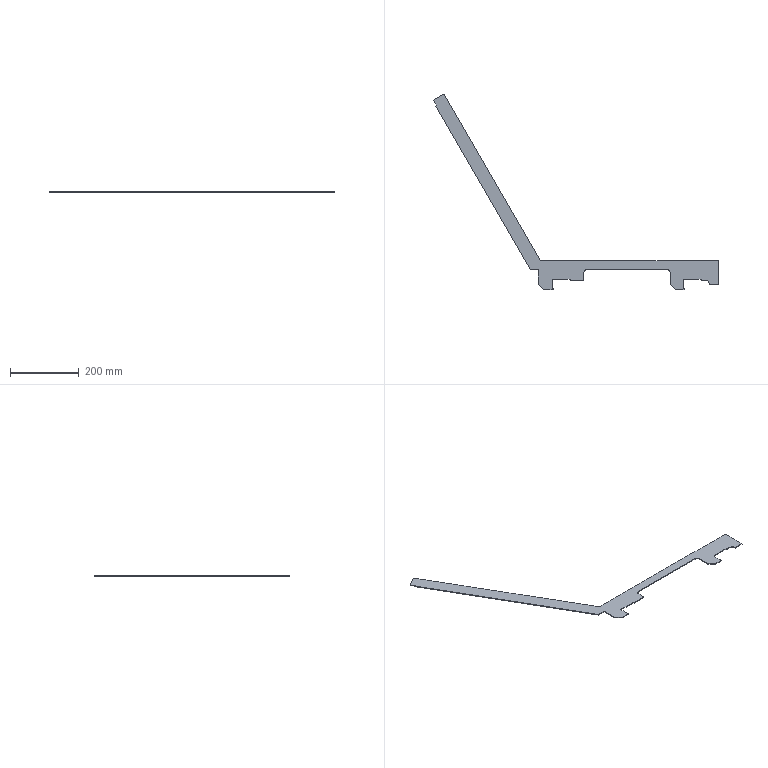Part | STEP file | zq001-1 | 1 solid | 37 faces | box 827.736 x 568.376 x 2 mm | volume 90659 mm3 | plane 32 | cylinder 5 | commonest cylinder face diameters 20 x3 2 x2
STEP:
#1=CARTESIAN_POINT('',(-553.217,491.842,-2.));
#2=VERTEX_POINT('',#1);
#3=CARTESIAN_POINT('',(-544.917,477.466,-2.));
#4=VERTEX_POINT('',#3);
#5=CARTESIAN_POINT('',(-553.217,491.842,-2.));
#6=DIRECTION('',(0.5,-0.866,0.));
#7=VECTOR('',#6,1000.);
#8=LINE('',#5,#7);
#9=EDGE_CURVE('',#2,#4,#8,.T.);
#10=ORIENTED_EDGE('',*,*,#9,.F.);
#11=CARTESIAN_POINT('',(-523.079,509.242,-2.));
#12=VERTEX_POINT('',#11);
#13=CARTESIAN_POINT('',(-523.079,509.242,-2.));
#14=DIRECTION('',(-0.866,-0.5,0.));
#15=VECTOR('',#14,1000.);
#16=LINE('',#13,#15);
#17=EDGE_CURVE('',#12,#2,#16,.T.);
#18=ORIENTED_EDGE('',*,*,#17,.F.);
#19=CARTESIAN_POINT('',(-521.713,508.876,-2.));
#20=VERTEX_POINT('',#19);
#21=CARTESIAN_POINT('',(-522.579,508.376,-2.));
#22=DIRECTION('',(0.,0.,1.));
#23=DIRECTION('',(1.,0.,0.));
#24=AXIS2_PLACEMENT_3D('',#21,#22,#23);
#25=CIRCLE('',#24,1.);
#26=EDGE_CURVE('',#20,#12,#25,.T.);
#27=ORIENTED_EDGE('',*,*,#26,.F.);
#28=CARTESIAN_POINT('',(-242.636,25.5,-2.));
#29=VERTEX_POINT('',#28);
#30=CARTESIAN_POINT('',(-242.636,25.5,-2.));
#31=DIRECTION('',(-0.5,0.866,0.));
#32=VECTOR('',#31,1000.);
#33=LINE('',#30,#32);
#34=EDGE_CURVE('',#29,#20,#33,.T.);
#35=ORIENTED_EDGE('',*,*,#34,.F.);
#36=CARTESIAN_POINT('',(273.519,25.5,-2.));
#37=VERTEX_POINT('',#36);
#38=CARTESIAN_POINT('',(-522.579,25.5,-2.));
#39=DIRECTION('',(-1.,0.,0.));
#40=VECTOR('',#39,1000.);
#41=LINE('',#38,#40);
#42=EDGE_CURVE('',#37,#29,#41,.T.);
#43=ORIENTED_EDGE('',*,*,#42,.F.);
#44=CARTESIAN_POINT('',(274.519,24.5,-2.));
#45=VERTEX_POINT('',#44);
#46=CARTESIAN_POINT('',(273.519,24.5,-2.));
#47=DIRECTION('',(0.,0.,1.));
#48=DIRECTION('',(1.,0.,0.));
#49=AXIS2_PLACEMENT_3D('',#46,#47,#48);
#50=CIRCLE('',#49,1.);
#51=EDGE_CURVE('',#45,#37,#50,.T.);
#52=ORIENTED_EDGE('',*,*,#51,.F.);
#53=CARTESIAN_POINT('',(274.519,-42.5,-2.));
#54=VERTEX_POINT('',#53);
#55=CARTESIAN_POINT('',(274.519,508.376,-2.));
#56=DIRECTION('',(0.,1.,0.));
#57=VECTOR('',#56,1000.);
#58=LINE('',#55,#57);
#59=EDGE_CURVE('',#54,#45,#58,.T.);
#60=ORIENTED_EDGE('',*,*,#59,.F.);
#61=CARTESIAN_POINT('',(246.519,-42.5,-2.));
#62=VERTEX_POINT('',#61);
#63=CARTESIAN_POINT('',(-522.579,-42.5,-2.));
#64=DIRECTION('',(1.,0.,0.));
#65=VECTOR('',#64,1000.);
#66=LINE('',#63,#65);
#67=EDGE_CURVE('',#62,#54,#66,.T.);
#68=ORIENTED_EDGE('',*,*,#67,.F.);
#69=CARTESIAN_POINT('',(246.519,-40.5,-2.));
#70=VERTEX_POINT('',#69);
#71=CARTESIAN_POINT('',(246.519,508.376,-2.));
#72=DIRECTION('',(0.,-1.,0.));
#73=VECTOR('',#72,1000.);
#74=LINE('',#71,#73);
#75=EDGE_CURVE('',#70,#62,#74,.T.);
#76=ORIENTED_EDGE('',*,*,#75,.F.);
#77=CARTESIAN_POINT('',(236.519,-30.5,-2.));
#78=VERTEX_POINT('',#77);
#79=CARTESIAN_POINT('',(236.519,-40.5,-2.));
#80=DIRECTION('',(0.,0.,-1.));
#81=DIRECTION('',(1.,0.,0.));
#82=AXIS2_PLACEMENT_3D('',#79,#80,#81);
#83=CIRCLE('',#82,10.);
#84=EDGE_CURVE('',#78,#70,#83,.T.);
#85=ORIENTED_EDGE('',*,*,#84,.F.);
#86=CARTESIAN_POINT('',(223.519,-30.5,-2.));
#87=VERTEX_POINT('',#86);
#88=CARTESIAN_POINT('',(-522.579,-30.5,-2.));
#89=DIRECTION('',(1.,0.,0.));
#90=VECTOR('',#89,1000.);
#91=LINE('',#88,#90);
#92=EDGE_CURVE('',#87,#78,#91,.T.);
#93=ORIENTED_EDGE('',*,*,#92,.F.);
#94=CARTESIAN_POINT('',(223.519,-28.,-2.));
#95=VERTEX_POINT('',#94);
#96=CARTESIAN_POINT('',(223.519,508.376,-2.));
#97=DIRECTION('',(0.,-1.,0.));
#98=VECTOR('',#97,1000.);
#99=LINE('',#96,#98);
#100=EDGE_CURVE('',#95,#87,#99,.T.);
#101=ORIENTED_EDGE('',*,*,#100,.F.);
#102=CARTESIAN_POINT('',(171.519,-28.,-2.));
#103=VERTEX_POINT('',#102);
#104=CARTESIAN_POINT('',(-522.579,-28.,-2.));
#105=DIRECTION('',(1.,0.,0.));
#106=VECTOR('',#105,1000.);
#107=LINE('',#104,#106);
#108=EDGE_CURVE('',#103,#95,#107,.T.);
#109=ORIENTED_EDGE('',*,*,#108,.F.);
#110=CARTESIAN_POINT('',(171.519,-56.,-2.));
#111=VERTEX_POINT('',#110);
#112=CARTESIAN_POINT('',(171.519,508.376,-2.));
#113=DIRECTION('',(0.,1.,0.));
#114=VECTOR('',#113,1000.);
#115=LINE('',#112,#114);
#116=EDGE_CURVE('',#111,#103,#115,.T.);
#117=ORIENTED_EDGE('',*,*,#116,.F.);
#118=CARTESIAN_POINT('',(174.019,-56.,-2.));
#119=VERTEX_POINT('',#118);
#120=CARTESIAN_POINT('',(-522.579,-56.,-2.));
#121=DIRECTION('',(-1.,0.,0.));
#122=VECTOR('',#121,1000.);
#123=LINE('',#120,#122);
#124=EDGE_CURVE('',#119,#111,#123,.T.);
#125=ORIENTED_EDGE('',*,*,#124,.F.);
#126=CARTESIAN_POINT('',(174.019,-59.,-2.));
#127=VERTEX_POINT('',#126);
#128=CARTESIAN_POINT('',(174.019,508.376,-2.));
#129=DIRECTION('',(0.,1.,0.));
#130=VECTOR('',#129,1000.);
#131=LINE('',#128,#130);
#132=EDGE_CURVE('',#127,#119,#131,.T.);
#133=ORIENTED_EDGE('',*,*,#132,.F.);
#134=CARTESIAN_POINT('',(150.019,-59.,-2.));
#135=VERTEX_POINT('',#134);
#136=CARTESIAN_POINT('',(-522.579,-59.,-2.));
#137=DIRECTION('',(1.,0.,0.));
#138=VECTOR('',#137,1000.);
#139=LINE('',#136,#138);
#140=EDGE_CURVE('',#135,#127,#139,.T.);
#141=ORIENTED_EDGE('',*,*,#140,.F.);
#142=CARTESIAN_POINT('',(134.019,-43.,-2.));
#143=VERTEX_POINT('',#142);
#144=CARTESIAN_POINT('',(134.019,-43.,-2.));
#145=DIRECTION('',(0.7071,-0.7071,0.));
#146=VECTOR('',#145,1000.);
#147=LINE('',#144,#146);
#148=EDGE_CURVE('',#143,#135,#147,.T.);
#149=ORIENTED_EDGE('',*,*,#148,.F.);
#150=CARTESIAN_POINT('',(134.019,-10.,-2.));
#151=VERTEX_POINT('',#150);
#152=CARTESIAN_POINT('',(134.019,508.376,-2.));
#153=DIRECTION('',(0.,-1.,0.));
#154=VECTOR('',#153,1000.);
#155=LINE('',#152,#154);
#156=EDGE_CURVE('',#151,#143,#155,.T.);
#157=ORIENTED_EDGE('',*,*,#156,.F.);
#158=CARTESIAN_POINT('',(124.019,0.,-2.));
#159=VERTEX_POINT('',#158);
#160=CARTESIAN_POINT('',(124.019,-10.,-2.));
#161=DIRECTION('',(0.,0.,-1.));
#162=DIRECTION('',(1.,0.,0.));
#163=AXIS2_PLACEMENT_3D('',#160,#161,#162);
#164=CIRCLE('',#163,10.);
#165=EDGE_CURVE('',#159,#151,#164,.T.);
#166=ORIENTED_EDGE('',*,*,#165,.F.);
#167=CARTESIAN_POINT('',(-106.481,0.,-2.));
#168=VERTEX_POINT('',#167);
#169=CARTESIAN_POINT('',(-522.579,0.,-2.));
#170=DIRECTION('',(1.,0.,0.));
#171=VECTOR('',#170,1000.);
#172=LINE('',#169,#171);
#173=EDGE_CURVE('',#168,#159,#172,.T.);
#174=ORIENTED_EDGE('',*,*,#173,.F.);
#175=CARTESIAN_POINT('',(-116.481,-10.,-2.));
#176=VERTEX_POINT('',#175);
#177=CARTESIAN_POINT('',(-106.481,-10.,-2.));
#178=DIRECTION('',(0.,0.,-1.));
#179=DIRECTION('',(1.,0.,0.));
#180=AXIS2_PLACEMENT_3D('',#177,#178,#179);
#181=CIRCLE('',#180,10.);
#182=EDGE_CURVE('',#176,#168,#181,.T.);
#183=ORIENTED_EDGE('',*,*,#182,.F.);
#184=CARTESIAN_POINT('',(-116.481,-30.5,-2.));
#185=VERTEX_POINT('',#184);
#186=CARTESIAN_POINT('',(-116.481,508.376,-2.));
#187=DIRECTION('',(0.,1.,0.));
#188=VECTOR('',#187,1000.);
#189=LINE('',#186,#188);
#190=EDGE_CURVE('',#185,#176,#189,.T.);
#191=ORIENTED_EDGE('',*,*,#190,.F.);
#192=CARTESIAN_POINT('',(-156.481,-30.5,-2.));
#193=VERTEX_POINT('',#192);
#194=CARTESIAN_POINT('',(-522.579,-30.5,-2.));
#195=DIRECTION('',(1.,0.,0.));
#196=VECTOR('',#195,1000.);
#197=LINE('',#194,#196);
#198=EDGE_CURVE('',#193,#185,#197,.T.);
#199=ORIENTED_EDGE('',*,*,#198,.F.);
#200=CARTESIAN_POINT('',(-156.481,-28.,-2.));
#201=VERTEX_POINT('',#200);
#202=CARTESIAN_POINT('',(-156.481,508.376,-2.));
#203=DIRECTION('',(0.,-1.,0.));
#204=VECTOR('',#203,1000.);
#205=LINE('',#202,#204);
#206=EDGE_CURVE('',#201,#193,#205,.T.);
#207=ORIENTED_EDGE('',*,*,#206,.F.);
#208=CARTESIAN_POINT('',(-208.481,-28.,-2.));
#209=VERTEX_POINT('',#208);
#210=CARTESIAN_POINT('',(-522.579,-28.,-2.));
#211=DIRECTION('',(1.,0.,0.));
#212=VECTOR('',#211,1000.);
#213=LINE('',#210,#212);
#214=EDGE_CURVE('',#209,#201,#213,.T.);
#215=ORIENTED_EDGE('',*,*,#214,.F.);
#216=CARTESIAN_POINT('',(-208.481,-56.,-2.));
#217=VERTEX_POINT('',#216);
#218=CARTESIAN_POINT('',(-208.481,508.376,-2.));
#219=DIRECTION('',(0.,1.,0.));
#220=VECTOR('',#219,1000.);
#221=LINE('',#218,#220);
#222=EDGE_CURVE('',#217,#209,#221,.T.);
#223=ORIENTED_EDGE('',*,*,#222,.F.);
#224=CARTESIAN_POINT('',(-205.981,-56.,-2.));
#225=VERTEX_POINT('',#224);
#226=CARTESIAN_POINT('',(-522.579,-56.,-2.));
#227=DIRECTION('',(-1.,0.,0.));
#228=VECTOR('',#227,1000.);
#229=LINE('',#226,#228);
#230=EDGE_CURVE('',#225,#217,#229,.T.);
#231=ORIENTED_EDGE('',*,*,#230,.F.);
#232=CARTESIAN_POINT('',(-205.981,-59.,-2.));
#233=VERTEX_POINT('',#232);
#234=CARTESIAN_POINT('',(-205.981,508.376,-2.));
#235=DIRECTION('',(0.,1.,0.));
#236=VECTOR('',#235,1000.);
#237=LINE('',#234,#236);
#238=EDGE_CURVE('',#233,#225,#237,.T.);
#239=ORIENTED_EDGE('',*,*,#238,.F.);
#240=CARTESIAN_POINT('',(-232.481,-59.,-2.));
#241=VERTEX_POINT('',#240);
#242=CARTESIAN_POINT('',(-522.579,-59.,-2.));
#243=DIRECTION('',(1.,0.,0.));
#244=VECTOR('',#243,1000.);
#245=LINE('',#242,#244);
#246=EDGE_CURVE('',#241,#233,#245,.T.);
#247=ORIENTED_EDGE('',*,*,#246,.F.);
#248=CARTESIAN_POINT('',(-248.481,-43.,-2.));
#249=VERTEX_POINT('',#248);
#250=CARTESIAN_POINT('',(-248.481,-43.,-2.));
#251=DIRECTION('',(0.7071,-0.7071,0.));
#252=VECTOR('',#251,1000.);
#253=LINE('',#250,#252);
#254=EDGE_CURVE('',#249,#241,#253,.T.);
#255=ORIENTED_EDGE('',*,*,#254,.F.);
#256=CARTESIAN_POINT('',(-248.481,0.,-2.));
#257=VERTEX_POINT('',#256);
#258=CARTESIAN_POINT('',(-248.481,508.376,-2.));
#259=DIRECTION('',(0.,-1.,0.));
#260=VECTOR('',#259,1000.);
#261=LINE('',#258,#260);
#262=EDGE_CURVE('',#257,#249,#261,.T.);
#263=ORIENTED_EDGE('',*,*,#262,.F.);
#264=CARTESIAN_POINT('',(-271.792,0.,-2.));
#265=VERTEX_POINT('',#264);
#266=CARTESIAN_POINT('',(-522.579,0.,-2.));
#267=DIRECTION('',(1.,0.,0.));
#268=VECTOR('',#267,1000.);
#269=LINE('',#266,#268);
#270=EDGE_CURVE('',#265,#257,#269,.T.);
#271=ORIENTED_EDGE('',*,*,#270,.F.);
#272=CARTESIAN_POINT('',(-545.722,474.461,-2.));
#273=VERTEX_POINT('',#272);
#274=CARTESIAN_POINT('',(-545.722,474.461,-2.));
#275=DIRECTION('',(0.5,-0.866,0.));
#276=VECTOR('',#275,1000.);
#277=LINE('',#274,#276);
#278=EDGE_CURVE('',#273,#265,#277,.T.);
#279=ORIENTED_EDGE('',*,*,#278,.F.);
#280=CARTESIAN_POINT('',(-544.917,477.466,-2.));
#281=DIRECTION('',(-0.2588,-0.9659,0.));
#282=VECTOR('',#281,1000.);
#283=LINE('',#280,#282);
#284=EDGE_CURVE('',#4,#273,#283,.T.);
#285=ORIENTED_EDGE('',*,*,#284,.F.);
#286=EDGE_LOOP('',(#10,#18,#27,#35,#43,#52,#60,#68,#76,#85,#93,#101,#109,#117,#125,#133,#141,#149,#157,#166,#174,#183,#191,#199,#207,#215,#223,#231,#239,#247,#255,#263,#271,#279,#285));
#287=FACE_OUTER_BOUND('',#286,.T.);
#288=CARTESIAN_POINT('',(-522.579,508.376,-2.));
#289=DIRECTION('',(0.,0.,1.));
#290=DIRECTION('',(1.,0.,0.));
#291=AXIS2_PLACEMENT_3D('',#288,#289,#290);
#292=PLANE('',#291);
#293=ADVANCED_FACE('',(#287),#292,.F.);
#294=CARTESIAN_POINT('',(-545.722,474.461,0.));
#295=VERTEX_POINT('',#294);
#296=CARTESIAN_POINT('',(-545.722,474.461,-2.));
#297=DIRECTION('',(0.,0.,-1.));
#298=VECTOR('',#297,1000.);
#299=LINE('',#296,#298);
#300=EDGE_CURVE('',#295,#273,#299,.T.);
#301=ORIENTED_EDGE('',*,*,#300,.F.);
#302=CARTESIAN_POINT('',(-544.917,477.466,0.));
#303=VERTEX_POINT('',#302);
#304=CARTESIAN_POINT('',(-544.88,477.603,0.));
#305=DIRECTION('',(-0.2588,-0.9659,0.));
#306=VECTOR('',#305,1000.);
#307=LINE('',#304,#306);
#308=EDGE_CURVE('',#303,#295,#307,.T.);
#309=ORIENTED_EDGE('',*,*,#308,.F.);
#310=CARTESIAN_POINT('',(-544.917,477.466,-2.));
#311=DIRECTION('',(0.,0.,1.));
#312=VECTOR('',#311,1000.);
#313=LINE('',#310,#312);
#314=EDGE_CURVE('',#4,#303,#313,.T.);
#315=ORIENTED_EDGE('',*,*,#314,.F.);
#316=ORIENTED_EDGE('',*,*,#284,.T.);
#317=EDGE_LOOP('',(#301,#309,#315,#316));
#318=FACE_OUTER_BOUND('',#317,.T.);
#319=CARTESIAN_POINT('',(-544.88,477.603,-2.));
#320=DIRECTION('',(0.9659,-0.2588,0.));
#321=DIRECTION('',(0.2588,0.9659,0.));
#322=AXIS2_PLACEMENT_3D('',#319,#320,#321);
#323=PLANE('',#322);
#324=ADVANCED_FACE('',(#318),#323,.F.);
#325=ORIENTED_EDGE('',*,*,#9,.T.);
#326=ORIENTED_EDGE('',*,*,#314,.T.);
#327=CARTESIAN_POINT('',(-553.217,491.842,0.));
#328=VERTEX_POINT('',#327);
#329=CARTESIAN_POINT('',(-553.217,491.842,0.));
#330=DIRECTION('',(-0.5,0.866,0.));
#331=VECTOR('',#330,1000.);
#332=LINE('',#329,#331);
#333=EDGE_CURVE('',#303,#328,#332,.T.);
#334=ORIENTED_EDGE('',*,*,#333,.T.);
#335=CARTESIAN_POINT('',(-553.217,491.842,-2.));
#336=DIRECTION('',(0.,0.,-1.));
#337=VECTOR('',#336,1000.);
#338=LINE('',#335,#337);
#339=EDGE_CURVE('',#328,#2,#338,.T.);
#340=ORIENTED_EDGE('',*,*,#339,.T.);
#341=EDGE_LOOP('',(#325,#326,#334,#340));
#342=FACE_OUTER_BOUND('',#341,.T.);
#343=CARTESIAN_POINT('',(-553.217,491.842,-2.));
#344=DIRECTION('',(-0.866,-0.5,0.));
#345=DIRECTION('',(0.5,-0.866,0.));
#346=AXIS2_PLACEMENT_3D('',#343,#344,#345);
#347=PLANE('',#346);
#348=ADVANCED_FACE('',(#342),#347,.T.);
#349=ORIENTED_EDGE('',*,*,#17,.T.);
#350=ORIENTED_EDGE('',*,*,#339,.F.);
#351=CARTESIAN_POINT('',(-523.079,509.242,0.));
#352=VERTEX_POINT('',#351);
#353=CARTESIAN_POINT('',(-523.079,509.242,0.));
#354=DIRECTION('',(0.866,0.5,0.));
#355=VECTOR('',#354,1000.);
#356=LINE('',#353,#355);
#357=EDGE_CURVE('',#328,#352,#356,.T.);
#358=ORIENTED_EDGE('',*,*,#357,.T.);
#359=CARTESIAN_POINT('',(-523.079,509.242,-2.));
#360=DIRECTION('',(0.,0.,-1.));
#361=VECTOR('',#360,1000.);
#362=LINE('',#359,#361);
#363=EDGE_CURVE('',#352,#12,#362,.T.);
#364=ORIENTED_EDGE('',*,*,#363,.T.);
#365=EDGE_LOOP('',(#349,#350,#358,#364));
#366=FACE_OUTER_BOUND('',#365,.T.);
#367=CARTESIAN_POINT('',(-523.079,509.242,-2.));
#368=DIRECTION('',(-0.5,0.866,0.));
#369=DIRECTION('',(-0.866,-0.5,0.));
#370=AXIS2_PLACEMENT_3D('',#367,#368,#369);
#371=PLANE('',#370);
#372=ADVANCED_FACE('',(#366),#371,.T.);
#373=ORIENTED_EDGE('',*,*,#34,.T.);
#374=CARTESIAN_POINT('',(-521.713,508.876,0.));
#375=VERTEX_POINT('',#374);
#376=CARTESIAN_POINT('',(-521.713,508.876,-2.));
#377=DIRECTION('',(0.,0.,1.));
#378=VECTOR('',#377,1000.);
#379=LINE('',#376,#378);
#380=EDGE_CURVE('',#20,#375,#379,.T.);
#381=ORIENTED_EDGE('',*,*,#380,.T.);
#382=CARTESIAN_POINT('',(-242.636,25.5,0.));
#383=VERTEX_POINT('',#382);
#384=CARTESIAN_POINT('',(-242.636,25.5,0.));
#385=DIRECTION('',(0.5,-0.866,0.));
#386=VECTOR('',#385,1000.);
#387=LINE('',#384,#386);
#388=EDGE_CURVE('',#375,#383,#387,.T.);
#389=ORIENTED_EDGE('',*,*,#388,.T.);
#390=CARTESIAN_POINT('',(-242.636,25.5,-2.));
#391=DIRECTION('',(0.,0.,-1.));
#392=VECTOR('',#391,1000.);
#393=LINE('',#390,#392);
#394=EDGE_CURVE('',#383,#29,#393,.T.);
#395=ORIENTED_EDGE('',*,*,#394,.T.);
#396=EDGE_LOOP('',(#373,#381,#389,#395));
#397=FACE_OUTER_BOUND('',#396,.T.);
#398=CARTESIAN_POINT('',(-242.636,25.5,-2.));
#399=DIRECTION('',(0.866,0.5,0.));
#400=DIRECTION('',(-0.5,0.866,0.));
#401=AXIS2_PLACEMENT_3D('',#398,#399,#400);
#402=PLANE('',#401);
#403=ADVANCED_FACE('',(#397),#402,.T.);
#404=ORIENTED_EDGE('',*,*,#42,.T.);
#405=ORIENTED_EDGE('',*,*,#394,.F.);
#406=CARTESIAN_POINT('',(273.519,25.5,0.));
#407=VERTEX_POINT('',#406);
#408=CARTESIAN_POINT('',(273.519,25.5,0.));
#409=DIRECTION('',(1.,0.,0.));
#410=VECTOR('',#409,1000.);
#411=LINE('',#408,#410);
#412=EDGE_CURVE('',#383,#407,#411,.T.);
#413=ORIENTED_EDGE('',*,*,#412,.T.);
#414=CARTESIAN_POINT('',(273.519,25.5,-2.));
#415=DIRECTION('',(0.,0.,-1.));
#416=VECTOR('',#415,1000.);
#417=LINE('',#414,#416);
#418=EDGE_CURVE('',#407,#37,#417,.T.);
#419=ORIENTED_EDGE('',*,*,#418,.T.);
#420=EDGE_LOOP('',(#404,#405,#413,#419));
#421=FACE_OUTER_BOUND('',#420,.T.);
#422=CARTESIAN_POINT('',(273.519,25.5,-2.));
#423=DIRECTION('',(0.,1.,0.));
#424=DIRECTION('',(-1.,0.,0.));
#425=AXIS2_PLACEMENT_3D('',#422,#423,#424);
#426=PLANE('',#425);
#427=ADVANCED_FACE('',(#421),#426,.T.);
#428=ORIENTED_EDGE('',*,*,#59,.T.);
#429=CARTESIAN_POINT('',(274.519,24.5,0.));
#430=VERTEX_POINT('',#429);
#431=CARTESIAN_POINT('',(274.519,24.5,-2.));
#432=DIRECTION('',(0.,0.,1.));
#433=VECTOR('',#432,1000.);
#434=LINE('',#431,#433);
#435=EDGE_CURVE('',#45,#430,#434,.T.);
#436=ORIENTED_EDGE('',*,*,#435,.T.);
#437=CARTESIAN_POINT('',(274.519,-42.5,0.));
#438=VERTEX_POINT('',#437);
#439=CARTESIAN_POINT('',(274.519,-42.5,0.));
#440=DIRECTION('',(0.,-1.,0.));
#441=VECTOR('',#440,1000.);
#442=LINE('',#439,#441);
#443=EDGE_CURVE('',#430,#438,#442,.T.);
#444=ORIENTED_EDGE('',*,*,#443,.T.);
#445=CARTESIAN_POINT('',(274.519,-42.5,-2.));
#446=DIRECTION('',(0.,0.,-1.));
#447=VECTOR('',#446,1000.);
#448=LINE('',#445,#447);
#449=EDGE_CURVE('',#438,#54,#448,.T.);
#450=ORIENTED_EDGE('',*,*,#449,.T.);
#451=EDGE_LOOP('',(#428,#436,#444,#450));
#452=FACE_OUTER_BOUND('',#451,.T.);
#453=CARTESIAN_POINT('',(274.519,-42.5,-2.));
#454=DIRECTION('',(1.,0.,0.));
#455=DIRECTION('',(0.,0.,-1.));
#456=AXIS2_PLACEMENT_3D('',#453,#454,#455);
#457=PLANE('',#456);
#458=ADVANCED_FACE('',(#452),#457,.T.);
#459=ORIENTED_EDGE('',*,*,#67,.T.);
#460=ORIENTED_EDGE('',*,*,#449,.F.);
#461=CARTESIAN_POINT('',(246.519,-42.5,0.));
#462=VERTEX_POINT('',#461);
#463=CARTESIAN_POINT('',(246.519,-42.5,0.));
#464=DIRECTION('',(-1.,0.,0.));
#465=VECTOR('',#464,1000.);
#466=LINE('',#463,#465);
#467=EDGE_CURVE('',#438,#462,#466,.T.);
#468=ORIENTED_EDGE('',*,*,#467,.T.);
#469=CARTESIAN_POINT('',(246.519,-42.5,-2.));
#470=DIRECTION('',(0.,0.,-1.));
#471=VECTOR('',#470,1000.);
#472=LINE('',#469,#471);
#473=EDGE_CURVE('',#462,#62,#472,.T.);
#474=ORIENTED_EDGE('',*,*,#473,.T.);
#475=EDGE_LOOP('',(#459,#460,#468,#474));
#476=FACE_OUTER_BOUND('',#475,.T.);
#477=CARTESIAN_POINT('',(246.519,-42.5,-2.));
#478=DIRECTION('',(0.,-1.,0.));
#479=DIRECTION('',(1.,0.,0.));
#480=AXIS2_PLACEMENT_3D('',#477,#478,#479);
#481=PLANE('',#480);
#482=ADVANCED_FACE('',(#476),#481,.T.);
#483=ORIENTED_EDGE('',*,*,#75,.T.);
#484=ORIENTED_EDGE('',*,*,#473,.F.);
#485=CARTESIAN_POINT('',(246.519,-40.5,0.));
#486=VERTEX_POINT('',#485);
#487=CARTESIAN_POINT('',(246.519,-40.5,0.));
#488=DIRECTION('',(0.,1.,0.));
#489=VECTOR('',#488,1000.);
#490=LINE('',#487,#489);
#491=EDGE_CURVE('',#462,#486,#490,.T.);
#492=ORIENTED_EDGE('',*,*,#491,.T.);
#493=CARTESIAN_POINT('',(246.519,-40.5,-2.));
#494=DIRECTION('',(0.,0.,-1.));
#495=VECTOR('',#494,1000.);
#496=LINE('',#493,#495);
#497=EDGE_CURVE('',#486,#70,#496,.T.);
#498=ORIENTED_EDGE('',*,*,#497,.T.);
#499=EDGE_LOOP('',(#483,#484,#492,#498));
#500=FACE_OUTER_BOUND('',#499,.T.);
#501=CARTESIAN_POINT('',(246.519,-40.5,-2.));
#502=DIRECTION('',(-1.,0.,0.));
#503=DIRECTION('',(0.,0.,1.));
#504=AXIS2_PLACEMENT_3D('',#501,#502,#503);
#505=PLANE('',#504);
#506=ADVANCED_FACE('',(#500),#505,.T.);
#507=CARTESIAN_POINT('',(236.519,-30.5,0.));
#508=VERTEX_POINT('',#507);
#509=CARTESIAN_POINT('',(236.519,-30.5,-2.));
#510=DIRECTION('',(0.,0.,1.));
#511=VECTOR('',#510,1000.);
#512=LINE('',#509,#511);
#513=EDGE_CURVE('',#78,#508,#512,.T.);
#514=ORIENTED_EDGE('',*,*,#513,.F.);
#515=ORIENTED_EDGE('',*,*,#84,.T.);
#516=ORIENTED_EDGE('',*,*,#497,.F.);
#517=CARTESIAN_POINT('',(236.519,-40.5,0.));
#518=DIRECTION('',(0.,0.,-1.));
#519=DIRECTION('',(1.,0.,0.));
#520=AXIS2_PLACEMENT_3D('',#517,#518,#519);
#521=CIRCLE('',#520,10.);
#522=EDGE_CURVE('',#508,#486,#521,.T.);
#523=ORIENTED_EDGE('',*,*,#522,.F.);
#524=EDGE_LOOP('',(#514,#515,#516,#523));
#525=FACE_OUTER_BOUND('',#524,.T.);
#526=CARTESIAN_POINT('',(236.519,-40.5,-2.));
#527=DIRECTION('',(0.,0.,1.));
#528=DIRECTION('',(1.,0.,0.));
#529=AXIS2_PLACEMENT_3D('',#526,#527,#528);
#530=CYLINDRICAL_SURFACE('',#529,10.);
#531=ADVANCED_FACE('',(#525),#530,.F.);
#532=ORIENTED_EDGE('',*,*,#92,.T.);
#533=ORIENTED_EDGE('',*,*,#513,.T.);
#534=CARTESIAN_POINT('',(223.519,-30.5,0.));
#535=VERTEX_POINT('',#534);
#536=CARTESIAN_POINT('',(223.519,-30.5,0.));
#537=DIRECTION('',(-1.,0.,0.));
#538=VECTOR('',#537,1000.);
#539=LINE('',#536,#538);
#540=EDGE_CURVE('',#508,#535,#539,.T.);
#541=ORIENTED_EDGE('',*,*,#540,.T.);
#542=CARTESIAN_POINT('',(223.519,-30.5,-2.));
#543=DIRECTION('',(0.,0.,-1.));
#544=VECTOR('',#543,1000.);
#545=LINE('',#542,#544);
#546=EDGE_CURVE('',#535,#87,#545,.T.);
#547=ORIENTED_EDGE('',*,*,#546,.T.);
#548=EDGE_LOOP('',(#532,#533,#541,#547));
#549=FACE_OUTER_BOUND('',#548,.T.);
#550=CARTESIAN_POINT('',(223.519,-30.5,-2.));
#551=DIRECTION('',(0.,-1.,0.));
#552=DIRECTION('',(1.,0.,0.));
#553=AXIS2_PLACEMENT_3D('',#550,#551,#552);
#554=PLANE('',#553);
#555=ADVANCED_FACE('',(#549),#554,.T.);
#556=ORIENTED_EDGE('',*,*,#100,.T.);
#557=ORIENTED_EDGE('',*,*,#546,.F.);
#558=CARTESIAN_POINT('',(223.519,-28.,0.));
#559=VERTEX_POINT('',#558);
#560=CARTESIAN_POINT('',(223.519,-28.,0.));
#561=DIRECTION('',(0.,1.,0.));
#562=VECTOR('',#561,1000.);
#563=LINE('',#560,#562);
#564=EDGE_CURVE('',#535,#559,#563,.T.);
#565=ORIENTED_EDGE('',*,*,#564,.T.);
#566=CARTESIAN_POINT('',(223.519,-28.,-2.));
#567=DIRECTION('',(0.,0.,-1.));
#568=VECTOR('',#567,1000.);
#569=LINE('',#566,#568);
#570=EDGE_CURVE('',#559,#95,#569,.T.);
#571=ORIENTED_EDGE('',*,*,#570,.T.);
#572=EDGE_LOOP('',(#556,#557,#565,#571));
#573=FACE_OUTER_BOUND('',#572,.T.);
#574=CARTESIAN_POINT('',(223.519,-28.,-2.));
#575=DIRECTION('',(-1.,0.,0.));
#576=DIRECTION('',(0.,-1.,0.));
#577=AXIS2_PLACEMENT_3D('',#574,#575,#576);
#578=PLANE('',#577);
#579=ADVANCED_FACE('',(#573),#578,.T.);
#580=ORIENTED_EDGE('',*,*,#108,.T.);
#581=ORIENTED_EDGE('',*,*,#570,.F.);
#582=CARTESIAN_POINT('',(171.519,-28.,0.));
#583=VERTEX_POINT('',#582);
#584=CARTESIAN_POINT('',(171.519,-28.,0.));
#585=DIRECTION('',(-1.,0.,0.));
#586=VECTOR('',#585,1000.);
#587=LINE('',#584,#586);
#588=EDGE_CURVE('',#559,#583,#587,.T.);
#589=ORIENTED_EDGE('',*,*,#588,.T.);
#590=CARTESIAN_POINT('',(171.519,-28.,-2.));
#591=DIRECTION('',(0.,0.,-1.));
#592=VECTOR('',#591,1000.);
#593=LINE('',#590,#592);
#594=EDGE_CURVE('',#583,#103,#593,.T.);
#595=ORIENTED_EDGE('',*,*,#594,.T.);
#596=EDGE_LOOP('',(#580,#581,#589,#595));
#597=FACE_OUTER_BOUND('',#596,.T.);
#598=CARTESIAN_POINT('',(171.519,-28.,-2.));
#599=DIRECTION('',(0.,-1.,0.));
#600=DIRECTION('',(1.,0.,0.));
#601=AXIS2_PLACEMENT_3D('',#598,#599,#600);
#602=PLANE('',#601);
#603=ADVANCED_FACE('',(#597),#602,.T.);
#604=ORIENTED_EDGE('',*,*,#116,.T.);
#605=ORIENTED_EDGE('',*,*,#594,.F.);
#606=CARTESIAN_POINT('',(171.519,-56.,0.));
#607=VERTEX_POINT('',#606);
#608=CARTESIAN_POINT('',(171.519,-56.,0.));
#609=DIRECTION('',(0.,-1.,0.));
#610=VECTOR('',#609,1000.);
#611=LINE('',#608,#610);
#612=EDGE_CURVE('',#583,#607,#611,.T.);
#613=ORIENTED_EDGE('',*,*,#612,.T.);
#614=CARTESIAN_POINT('',(171.519,-56.,-2.));
#615=DIRECTION('',(0.,0.,-1.));
#616=VECTOR('',#615,1000.);
#617=LINE('',#614,#616);
#618=EDGE_CURVE('',#607,#111,#617,.T.);
#619=ORIENTED_EDGE('',*,*,#618,.T.);
#620=EDGE_LOOP('',(#604,#605,#613,#619));
#621=FACE_OUTER_BOUND('',#620,.T.);
#622=CARTESIAN_POINT('',(171.519,-56.,-2.));
#623=DIRECTION('',(1.,0.,0.));
#624=DIRECTION('',(0.,1.,0.));
#625=AXIS2_PLACEMENT_3D('',#622,#623,#624);
#626=PLANE('',#625);
#627=ADVANCED_FACE('',(#621),#626,.T.);
#628=ORIENTED_EDGE('',*,*,#124,.T.);
#629=ORIENTED_EDGE('',*,*,#618,.F.);
#630=CARTESIAN_POINT('',(174.019,-56.,0.));
#631=VERTEX_POINT('',#630);
#632=CARTESIAN_POINT('',(171.519,-56.,0.));
#633=DIRECTION('',(1.,0.,0.));
#634=VECTOR('',#633,1000.);
#635=LINE('',#632,#634);
#636=EDGE_CURVE('',#607,#631,#635,.T.);
#637=ORIENTED_EDGE('',*,*,#636,.T.);
#638=CARTESIAN_POINT('',(174.019,-56.,-2.));
#639=DIRECTION('',(0.,0.,-1.));
#640=VECTOR('',#639,1000.);
#641=LINE('',#638,#640);
#642=EDGE_CURVE('',#631,#119,#641,.T.);
#643=ORIENTED_EDGE('',*,*,#642,.T.);
#644=EDGE_LOOP('',(#628,#629,#637,#643));
#645=FACE_OUTER_BOUND('',#644,.T.);
#646=CARTESIAN_POINT('',(171.519,-56.,-2.));
#647=DIRECTION('',(0.,1.,0.));
#648=DIRECTION('',(-1.,0.,0.));
#649=AXIS2_PLACEMENT_3D('',#646,#647,#648);
#650=PLANE('',#649);
#651=ADVANCED_FACE('',(#645),#650,.T.);
#652=ORIENTED_EDGE('',*,*,#132,.T.);
#653=ORIENTED_EDGE('',*,*,#642,.F.);
#654=CARTESIAN_POINT('',(174.019,-59.,0.));
#655=VERTEX_POINT('',#654);
#656=CARTESIAN_POINT('',(174.019,-56.,0.));
#657=DIRECTION('',(0.,-1.,0.));
#658=VECTOR('',#657,1000.);
#659=LINE('',#656,#658);
#660=EDGE_CURVE('',#631,#655,#659,.T.);
#661=ORIENTED_EDGE('',*,*,#660,.T.);
#662=CARTESIAN_POINT('',(174.019,-59.,-2.));
#663=DIRECTION('',(0.,0.,-1.));
#664=VECTOR('',#663,1000.);
#665=LINE('',#662,#664);
#666=EDGE_CURVE('',#655,#127,#665,.T.);
#667=ORIENTED_EDGE('',*,*,#666,.T.);
#668=EDGE_LOOP('',(#652,#653,#661,#667));
#669=FACE_OUTER_BOUND('',#668,.T.);
#670=CARTESIAN_POINT('',(174.019,-56.,-2.));
#671=DIRECTION('',(1.,0.,0.));
#672=DIRECTION('',(0.,0.,-1.));
#673=AXIS2_PLACEMENT_3D('',#670,#671,#672);
#674=PLANE('',#673);
#675=ADVANCED_FACE('',(#669),#674,.T.);
#676=ORIENTED_EDGE('',*,*,#140,.T.);
#677=ORIENTED_EDGE('',*,*,#666,.F.);
#678=CARTESIAN_POINT('',(150.019,-59.,0.));
#679=VERTEX_POINT('',#678);
#680=CARTESIAN_POINT('',(134.019,-59.,0.));
#681=DIRECTION('',(-1.,0.,0.));
#682=VECTOR('',#681,1000.);
#683=LINE('',#680,#682);
#684=EDGE_CURVE('',#655,#679,#683,.T.);
#685=ORIENTED_EDGE('',*,*,#684,.T.);
#686=CARTESIAN_POINT('',(150.019,-59.,-2.));
#687=DIRECTION('',(0.,0.,-1.));
#688=VECTOR('',#687,1000.);
#689=LINE('',#686,#688);
#690=EDGE_CURVE('',#679,#135,#689,.T.);
#691=ORIENTED_EDGE('',*,*,#690,.T.);
#692=EDGE_LOOP('',(#676,#677,#685,#691));
#693=FACE_OUTER_BOUND('',#692,.T.);
#694=CARTESIAN_POINT('',(134.019,-59.,-2.));
#695=DIRECTION('',(0.,-1.,0.));
#696=DIRECTION('',(1.,0.,0.));
#697=AXIS2_PLACEMENT_3D('',#694,#695,#696);
#698=PLANE('',#697);
#699=ADVANCED_FACE('',(#693),#698,.T.);
#700=ORIENTED_EDGE('',*,*,#690,.F.);
#701=CARTESIAN_POINT('',(134.019,-43.,0.));
#702=VERTEX_POINT('',#701);
#703=CARTESIAN_POINT('',(134.019,-43.,0.));
#704=DIRECTION('',(0.7071,-0.7071,0.));
#705=VECTOR('',#704,1000.);
#706=LINE('',#703,#705);
#707=EDGE_CURVE('',#702,#679,#706,.T.);
#708=ORIENTED_EDGE('',*,*,#707,.F.);
#709=CARTESIAN_POINT('',(134.019,-43.,-2.));
#710=DIRECTION('',(0.,0.,1.));
#711=VECTOR('',#710,1000.);
#712=LINE('',#709,#711);
#713=EDGE_CURVE('',#143,#702,#712,.T.);
#714=ORIENTED_EDGE('',*,*,#713,.F.);
#715=ORIENTED_EDGE('',*,*,#148,.T.);
#716=EDGE_LOOP('',(#700,#708,#714,#715));
#717=FACE_OUTER_BOUND('',#716,.T.);
#718=CARTESIAN_POINT('',(134.019,-43.,-2.));
#719=DIRECTION('',(0.7071,0.7071,0.));
#720=DIRECTION('',(-0.7071,0.7071,0.));
#721=AXIS2_PLACEMENT_3D('',#718,#719,#720);
#722=PLANE('',#721);
#723=ADVANCED_FACE('',(#717),#722,.F.);
#724=CARTESIAN_POINT('',(134.019,-10.,0.));
#725=VERTEX_POINT('',#724);
#726=CARTESIAN_POINT('',(134.019,-10.,0.));
#727=DIRECTION('',(0.,1.,0.));
#728=VECTOR('',#727,1000.);
#729=LINE('',#726,#728);
#730=EDGE_CURVE('',#702,#725,#729,.T.);
#731=ORIENTED_EDGE('',*,*,#730,.T.);
#732=CARTESIAN_POINT('',(134.019,-10.,-2.));
#733=DIRECTION('',(0.,0.,-1.));
#734=VECTOR('',#733,1000.);
#735=LINE('',#732,#734);
#736=EDGE_CURVE('',#725,#151,#735,.T.);
#737=ORIENTED_EDGE('',*,*,#736,.T.);
#738=ORIENTED_EDGE('',*,*,#156,.T.);
#739=ORIENTED_EDGE('',*,*,#713,.T.);
#740=EDGE_LOOP('',(#731,#737,#738,#739));
#741=FACE_OUTER_BOUND('',#740,.T.);
#742=CARTESIAN_POINT('',(134.019,-10.,-2.));
#743=DIRECTION('',(-1.,0.,0.));
#744=DIRECTION('',(0.,-1.,0.));
#745=AXIS2_PLACEMENT_3D('',#742,#743,#744);
#746=PLANE('',#745);
#747=ADVANCED_FACE('',(#741),#746,.T.);
#748=CARTESIAN_POINT('',(124.019,0.,0.));
#749=VERTEX_POINT('',#748);
#750=CARTESIAN_POINT('',(124.019,0.,-2.));
#751=DIRECTION('',(0.,0.,1.));
#752=VECTOR('',#751,1000.);
#753=LINE('',#750,#752);
#754=EDGE_CURVE('',#159,#749,#753,.T.);
#755=ORIENTED_EDGE('',*,*,#754,.F.);
#756=ORIENTED_EDGE('',*,*,#165,.T.);
#757=ORIENTED_EDGE('',*,*,#736,.F.);
#758=CARTESIAN_POINT('',(124.019,-10.,0.));
#759=DIRECTION('',(0.,0.,-1.));
#760=DIRECTION('',(1.,0.,0.));
#761=AXIS2_PLACEMENT_3D('',#758,#759,#760);
#762=CIRCLE('',#761,10.);
#763=EDGE_CURVE('',#749,#725,#762,.T.);
#764=ORIENTED_EDGE('',*,*,#763,.F.);
#765=EDGE_LOOP('',(#755,#756,#757,#764));
#766=FACE_OUTER_BOUND('',#765,.T.);
#767=CARTESIAN_POINT('',(124.019,-10.,-2.));
#768=DIRECTION('',(0.,0.,1.));
#769=DIRECTION('',(1.,0.,0.));
#770=AXIS2_PLACEMENT_3D('',#767,#768,#769);
#771=CYLINDRICAL_SURFACE('',#770,10.);
#772=ADVANCED_FACE('',(#766),#771,.F.);
#773=ORIENTED_EDGE('',*,*,#173,.T.);
#774=ORIENTED_EDGE('',*,*,#754,.T.);
#775=CARTESIAN_POINT('',(-106.481,0.,0.));
#776=VERTEX_POINT('',#775);
#777=CARTESIAN_POINT('',(-106.481,0.,0.));
#778=DIRECTION('',(-1.,0.,0.));
#779=VECTOR('',#778,1000.);
#780=LINE('',#777,#779);
#781=EDGE_CURVE('',#749,#776,#780,.T.);
#782=ORIENTED_EDGE('',*,*,#781,.T.);
#783=CARTESIAN_POINT('',(-106.481,0.,-2.));
#784=DIRECTION('',(0.,0.,-1.));
#785=VECTOR('',#784,1000.);
#786=LINE('',#783,#785);
#787=EDGE_CURVE('',#776,#168,#786,.T.);
#788=ORIENTED_EDGE('',*,*,#787,.T.);
#789=EDGE_LOOP('',(#773,#774,#782,#788));
#790=FACE_OUTER_BOUND('',#789,.T.);
#791=CARTESIAN_POINT('',(-106.481,0.,-2.));
#792=DIRECTION('',(0.,-1.,0.));
#793=DIRECTION('',(1.,0.,0.));
#794=AXIS2_PLACEMENT_3D('',#791,#792,#793);
#795=PLANE('',#794);
#796=ADVANCED_FACE('',(#790),#795,.T.);
#797=CARTESIAN_POINT('',(-116.481,-10.,0.));
#798=VERTEX_POINT('',#797);
#799=CARTESIAN_POINT('',(-116.481,-10.,-2.));
#800=DIRECTION('',(0.,0.,1.));
#801=VECTOR('',#800,1000.);
#802=LINE('',#799,#801);
#803=EDGE_CURVE('',#176,#798,#802,.T.);
#804=ORIENTED_EDGE('',*,*,#803,.F.);
#805=ORIENTED_EDGE('',*,*,#182,.T.);
#806=ORIENTED_EDGE('',*,*,#787,.F.);
#807=CARTESIAN_POINT('',(-106.481,-10.,0.));
#808=DIRECTION('',(0.,0.,-1.));
#809=DIRECTION('',(1.,0.,0.));
#810=AXIS2_PLACEMENT_3D('',#807,#808,#809);
#811=CIRCLE('',#810,10.);
#812=EDGE_CURVE('',#798,#776,#811,.T.);
#813=ORIENTED_EDGE('',*,*,#812,.F.);
#814=EDGE_LOOP('',(#804,#805,#806,#813));
#815=FACE_OUTER_BOUND('',#814,.T.);
#816=CARTESIAN_POINT('',(-106.481,-10.,-2.));
#817=DIRECTION('',(0.,0.,1.));
#818=DIRECTION('',(1.,0.,0.));
#819=AXIS2_PLACEMENT_3D('',#816,#817,#818);
#820=CYLINDRICAL_SURFACE('',#819,10.);
#821=ADVANCED_FACE('',(#815),#820,.F.);
#822=ORIENTED_EDGE('',*,*,#190,.T.);
#823=ORIENTED_EDGE('',*,*,#803,.T.);
#824=CARTESIAN_POINT('',(-116.481,-30.5,0.));
#825=VERTEX_POINT('',#824);
#826=CARTESIAN_POINT('',(-116.481,-30.5,0.));
#827=DIRECTION('',(0.,-1.,0.));
#828=VECTOR('',#827,1000.);
#829=LINE('',#826,#828);
#830=EDGE_CURVE('',#798,#825,#829,.T.);
#831=ORIENTED_EDGE('',*,*,#830,.T.);
#832=CARTESIAN_POINT('',(-116.481,-30.5,-2.));
#833=DIRECTION('',(0.,0.,-1.));
#834=VECTOR('',#833,1000.);
#835=LINE('',#832,#834);
#836=EDGE_CURVE('',#825,#185,#835,.T.);
#837=ORIENTED_EDGE('',*,*,#836,.T.);
#838=EDGE_LOOP('',(#822,#823,#831,#837));
#839=FACE_OUTER_BOUND('',#838,.T.);
#840=CARTESIAN_POINT('',(-116.481,-30.5,-2.));
#841=DIRECTION('',(1.,0.,0.));
#842=DIRECTION('',(0.,1.,0.));
#843=AXIS2_PLACEMENT_3D('',#840,#841,#842);
#844=PLANE('',#843);
#845=ADVANCED_FACE('',(#839),#844,.T.);
#846=ORIENTED_EDGE('',*,*,#198,.T.);
#847=ORIENTED_EDGE('',*,*,#836,.F.);
#848=CARTESIAN_POINT('',(-156.481,-30.5,0.));
#849=VERTEX_POINT('',#848);
#850=CARTESIAN_POINT('',(-156.481,-30.5,0.));
#851=DIRECTION('',(-1.,0.,0.));
#852=VECTOR('',#851,1000.);
#853=LINE('',#850,#852);
#854=EDGE_CURVE('',#825,#849,#853,.T.);
#855=ORIENTED_EDGE('',*,*,#854,.T.);
#856=CARTESIAN_POINT('',(-156.481,-30.5,-2.));
#857=DIRECTION('',(0.,0.,-1.));
#858=VECTOR('',#857,1000.);
#859=LINE('',#856,#858);
#860=EDGE_CURVE('',#849,#193,#859,.T.);
#861=ORIENTED_EDGE('',*,*,#860,.T.);
#862=EDGE_LOOP('',(#846,#847,#855,#861));
#863=FACE_OUTER_BOUND('',#862,.T.);
#864=CARTESIAN_POINT('',(-156.481,-30.5,-2.));
#865=DIRECTION('',(0.,-1.,0.));
#866=DIRECTION('',(1.,0.,0.));
#867=AXIS2_PLACEMENT_3D('',#864,#865,#866);
#868=PLANE('',#867);
#869=ADVANCED_FACE('',(#863),#868,.T.);
#870=ORIENTED_EDGE('',*,*,#206,.T.);
#871=ORIENTED_EDGE('',*,*,#860,.F.);
#872=CARTESIAN_POINT('',(-156.481,-28.,0.));
#873=VERTEX_POINT('',#872);
#874=CARTESIAN_POINT('',(-156.481,-28.,0.));
#875=DIRECTION('',(0.,1.,0.));
#876=VECTOR('',#875,1000.);
#877=LINE('',#874,#876);
#878=EDGE_CURVE('',#849,#873,#877,.T.);
#879=ORIENTED_EDGE('',*,*,#878,.T.);
#880=CARTESIAN_POINT('',(-156.481,-28.,-2.));
#881=DIRECTION('',(0.,0.,-1.));
#882=VECTOR('',#881,1000.);
#883=LINE('',#880,#882);
#884=EDGE_CURVE('',#873,#201,#883,.T.);
#885=ORIENTED_EDGE('',*,*,#884,.T.);
#886=EDGE_LOOP('',(#870,#871,#879,#885));
#887=FACE_OUTER_BOUND('',#886,.T.);
#888=CARTESIAN_POINT('',(-156.481,-28.,-2.));
#889=DIRECTION('',(-1.,0.,0.));
#890=DIRECTION('',(0.,-1.,0.));
#891=AXIS2_PLACEMENT_3D('',#888,#889,#890);
#892=PLANE('',#891);
#893=ADVANCED_FACE('',(#887),#892,.T.);
#894=ORIENTED_EDGE('',*,*,#214,.T.);
#895=ORIENTED_EDGE('',*,*,#884,.F.);
#896=CARTESIAN_POINT('',(-208.481,-28.,0.));
#897=VERTEX_POINT('',#896);
#898=CARTESIAN_POINT('',(-208.481,-28.,0.));
#899=DIRECTION('',(-1.,0.,0.));
#900=VECTOR('',#899,1000.);
#901=LINE('',#898,#900);
#902=EDGE_CURVE('',#873,#897,#901,.T.);
#903=ORIENTED_EDGE('',*,*,#902,.T.);
#904=CARTESIAN_POINT('',(-208.481,-28.,-2.));
#905=DIRECTION('',(0.,0.,-1.));
#906=VECTOR('',#905,1000.);
#907=LINE('',#904,#906);
#908=EDGE_CURVE('',#897,#209,#907,.T.);
#909=ORIENTED_EDGE('',*,*,#908,.T.);
#910=EDGE_LOOP('',(#894,#895,#903,#909));
#911=FACE_OUTER_BOUND('',#910,.T.);
#912=CARTESIAN_POINT('',(-208.481,-28.,-2.));
#913=DIRECTION('',(0.,-1.,0.));
#914=DIRECTION('',(1.,0.,0.));
#915=AXIS2_PLACEMENT_3D('',#912,#913,#914);
#916=PLANE('',#915);
#917=ADVANCED_FACE('',(#911),#916,.T.);
#918=ORIENTED_EDGE('',*,*,#222,.T.);
#919=ORIENTED_EDGE('',*,*,#908,.F.);
#920=CARTESIAN_POINT('',(-208.481,-56.,0.));
#921=VERTEX_POINT('',#920);
#922=CARTESIAN_POINT('',(-208.481,-56.,0.));
#923=DIRECTION('',(0.,-1.,0.));
#924=VECTOR('',#923,1000.);
#925=LINE('',#922,#924);
#926=EDGE_CURVE('',#897,#921,#925,.T.);
#927=ORIENTED_EDGE('',*,*,#926,.T.);
#928=CARTESIAN_POINT('',(-208.481,-56.,-2.));
#929=DIRECTION('',(0.,0.,-1.));
#930=VECTOR('',#929,1000.);
#931=LINE('',#928,#930);
#932=EDGE_CURVE('',#921,#217,#931,.T.);
#933=ORIENTED_EDGE('',*,*,#932,.T.);
#934=EDGE_LOOP('',(#918,#919,#927,#933));
#935=FACE_OUTER_BOUND('',#934,.T.);
#936=CARTESIAN_POINT('',(-208.481,-56.,-2.));
#937=DIRECTION('',(1.,0.,0.));
#938=DIRECTION('',(0.,1.,0.));
#939=AXIS2_PLACEMENT_3D('',#936,#937,#938);
#940=PLANE('',#939);
#941=ADVANCED_FACE('',(#935),#940,.T.);
#942=ORIENTED_EDGE('',*,*,#230,.T.);
#943=ORIENTED_EDGE('',*,*,#932,.F.);
#944=CARTESIAN_POINT('',(-205.981,-56.,0.));
#945=VERTEX_POINT('',#944);
#946=CARTESIAN_POINT('',(-208.481,-56.,0.));
#947=DIRECTION('',(1.,0.,0.));
#948=VECTOR('',#947,1000.);
#949=LINE('',#946,#948);
#950=EDGE_CURVE('',#921,#945,#949,.T.);
#951=ORIENTED_EDGE('',*,*,#950,.T.);
#952=CARTESIAN_POINT('',(-205.981,-56.,-2.));
#953=DIRECTION('',(0.,0.,-1.));
#954=VECTOR('',#953,1000.);
#955=LINE('',#952,#954);
#956=EDGE_CURVE('',#945,#225,#955,.T.);
#957=ORIENTED_EDGE('',*,*,#956,.T.);
#958=EDGE_LOOP('',(#942,#943,#951,#957));
#959=FACE_OUTER_BOUND('',#958,.T.);
#960=CARTESIAN_POINT('',(-208.481,-56.,-2.));
#961=DIRECTION('',(0.,1.,0.));
#962=DIRECTION('',(0.,0.,1.));
#963=AXIS2_PLACEMENT_3D('',#960,#961,#962);
#964=PLANE('',#963);
#965=ADVANCED_FACE('',(#959),#964,.T.);
#966=ORIENTED_EDGE('',*,*,#238,.T.);
#967=ORIENTED_EDGE('',*,*,#956,.F.);
#968=CARTESIAN_POINT('',(-205.981,-59.,0.));
#969=VERTEX_POINT('',#968);
#970=CARTESIAN_POINT('',(-205.981,-56.,0.));
#971=DIRECTION('',(0.,-1.,0.));
#972=VECTOR('',#971,1000.);
#973=LINE('',#970,#972);
#974=EDGE_CURVE('',#945,#969,#973,.T.);
#975=ORIENTED_EDGE('',*,*,#974,.T.);
#976=CARTESIAN_POINT('',(-205.981,-59.,-2.));
#977=DIRECTION('',(0.,0.,-1.));
#978=VECTOR('',#977,1000.);
#979=LINE('',#976,#978);
#980=EDGE_CURVE('',#969,#233,#979,.T.);
#981=ORIENTED_EDGE('',*,*,#980,.T.);
#982=EDGE_LOOP('',(#966,#967,#975,#981));
#983=FACE_OUTER_BOUND('',#982,.T.);
#984=CARTESIAN_POINT('',(-205.981,-56.,-2.));
#985=DIRECTION('',(1.,0.,0.));
#986=DIRECTION('',(0.,1.,0.));
#987=AXIS2_PLACEMENT_3D('',#984,#985,#986);
#988=PLANE('',#987);
#989=ADVANCED_FACE('',(#983),#988,.T.);
#990=ORIENTED_EDGE('',*,*,#246,.T.);
#991=ORIENTED_EDGE('',*,*,#980,.F.);
#992=CARTESIAN_POINT('',(-232.481,-59.,0.));
#993=VERTEX_POINT('',#992);
#994=CARTESIAN_POINT('',(-205.981,-59.,0.));
#995=DIRECTION('',(-1.,0.,0.));
#996=VECTOR('',#995,1000.);
#997=LINE('',#994,#996);
#998=EDGE_CURVE('',#969,#993,#997,.T.);
#999=ORIENTED_EDGE('',*,*,#998,.T.);
#1000=CARTESIAN_POINT('',(-232.481,-59.,-2.));
#1001=DIRECTION('',(0.,0.,-1.));
#1002=VECTOR('',#1001,1000.);
#1003=LINE('',#1000,#1002);
#1004=EDGE_CURVE('',#993,#241,#1003,.T.);
#1005=ORIENTED_EDGE('',*,*,#1004,.T.);
#1006=EDGE_LOOP('',(#990,#991,#999,#1005));
#1007=FACE_OUTER_BOUND('',#1006,.T.);
#1008=CARTESIAN_POINT('',(-205.981,-59.,-2.));
#1009=DIRECTION('',(0.,-1.,0.));
#1010=DIRECTION('',(1.,0.,0.));
#1011=AXIS2_PLACEMENT_3D('',#1008,#1009,#1010);
#1012=PLANE('',#1011);
#1013=ADVANCED_FACE('',(#1007),#1012,.T.);
#1014=ORIENTED_EDGE('',*,*,#1004,.F.);
#1015=CARTESIAN_POINT('',(-248.481,-43.,0.));
#1016=VERTEX_POINT('',#1015);
#1017=CARTESIAN_POINT('',(-248.481,-43.,0.));
#1018=DIRECTION('',(0.7071,-0.7071,0.));
#1019=VECTOR('',#1018,1000.);
#1020=LINE('',#1017,#1019);
#1021=EDGE_CURVE('',#1016,#993,#1020,.T.);
#1022=ORIENTED_EDGE('',*,*,#1021,.F.);
#1023=CARTESIAN_POINT('',(-248.481,-43.,-2.));
#1024=DIRECTION('',(0.,0.,1.));
#1025=VECTOR('',#1024,1000.);
#1026=LINE('',#1023,#1025);
#1027=EDGE_CURVE('',#249,#1016,#1026,.T.);
#1028=ORIENTED_EDGE('',*,*,#1027,.F.);
#1029=ORIENTED_EDGE('',*,*,#254,.T.);
#1030=EDGE_LOOP('',(#1014,#1022,#1028,#1029));
#1031=FACE_OUTER_BOUND('',#1030,.T.);
#1032=CARTESIAN_POINT('',(-248.481,-43.,-2.));
#1033=DIRECTION('',(0.7071,0.7071,0.));
#1034=DIRECTION('',(-0.7071,0.7071,0.));
#1035=AXIS2_PLACEMENT_3D('',#1032,#1033,#1034);
#1036=PLANE('',#1035);
#1037=ADVANCED_FACE('',(#1031),#1036,.F.);
#1038=CARTESIAN_POINT('',(-248.481,0.,0.));
#1039=VERTEX_POINT('',#1038);
#1040=CARTESIAN_POINT('',(-248.481,-59.,0.));
#1041=DIRECTION('',(0.,1.,0.));
#1042=VECTOR('',#1041,1000.);
#1043=LINE('',#1040,#1042);
#1044=EDGE_CURVE('',#1016,#1039,#1043,.T.);
#1045=ORIENTED_EDGE('',*,*,#1044,.T.);
#1046=CARTESIAN_POINT('',(-248.481,0.,-2.));
#1047=DIRECTION('',(0.,0.,-1.));
#1048=VECTOR('',#1047,1000.);
#1049=LINE('',#1046,#1048);
#1050=EDGE_CURVE('',#1039,#257,#1049,.T.);
#1051=ORIENTED_EDGE('',*,*,#1050,.T.);
#1052=ORIENTED_EDGE('',*,*,#262,.T.);
#1053=ORIENTED_EDGE('',*,*,#1027,.T.);
#1054=EDGE_LOOP('',(#1045,#1051,#1052,#1053));
#1055=FACE_OUTER_BOUND('',#1054,.T.);
#1056=CARTESIAN_POINT('',(-248.481,-59.,-2.));
#1057=DIRECTION('',(-1.,0.,0.));
#1058=DIRECTION('',(0.,0.,1.));
#1059=AXIS2_PLACEMENT_3D('',#1056,#1057,#1058);
#1060=PLANE('',#1059);
#1061=ADVANCED_FACE('',(#1055),#1060,.T.);
#1062=ORIENTED_EDGE('',*,*,#270,.T.);
#1063=ORIENTED_EDGE('',*,*,#1050,.F.);
#1064=CARTESIAN_POINT('',(-271.792,0.,0.));
#1065=VERTEX_POINT('',#1064);
#1066=CARTESIAN_POINT('',(-248.481,0.,0.));
#1067=DIRECTION('',(-1.,0.,0.));
#1068=VECTOR('',#1067,1000.);
#1069=LINE('',#1066,#1068);
#1070=EDGE_CURVE('',#1039,#1065,#1069,.T.);
#1071=ORIENTED_EDGE('',*,*,#1070,.T.);
#1072=CARTESIAN_POINT('',(-271.792,0.,-2.));
#1073=DIRECTION('',(0.,0.,-1.));
#1074=VECTOR('',#1073,1000.);
#1075=LINE('',#1072,#1074);
#1076=EDGE_CURVE('',#1065,#265,#1075,.T.);
#1077=ORIENTED_EDGE('',*,*,#1076,.T.);
#1078=EDGE_LOOP('',(#1062,#1063,#1071,#1077));
#1079=FACE_OUTER_BOUND('',#1078,.T.);
#1080=CARTESIAN_POINT('',(-248.481,0.,-2.));
#1081=DIRECTION('',(0.,-1.,0.));
#1082=DIRECTION('',(1.,0.,0.));
#1083=AXIS2_PLACEMENT_3D('',#1080,#1081,#1082);
#1084=PLANE('',#1083);
#1085=ADVANCED_FACE('',(#1079),#1084,.T.);
#1086=ORIENTED_EDGE('',*,*,#278,.T.);
#1087=ORIENTED_EDGE('',*,*,#1076,.F.);
#1088=CARTESIAN_POINT('',(-546.872,476.453,0.));
#1089=DIRECTION('',(-0.5,0.866,0.));
#1090=VECTOR('',#1089,1000.);
#1091=LINE('',#1088,#1090);
#1092=EDGE_CURVE('',#1065,#295,#1091,.T.);
#1093=ORIENTED_EDGE('',*,*,#1092,.T.);
#1094=ORIENTED_EDGE('',*,*,#300,.T.);
#1095=EDGE_LOOP('',(#1086,#1087,#1093,#1094));
#1096=FACE_OUTER_BOUND('',#1095,.T.);
#1097=CARTESIAN_POINT('',(-546.872,476.453,-2.));
#1098=DIRECTION('',(-0.866,-0.5,0.));
#1099=DIRECTION('',(0.5,-0.866,0.));
#1100=AXIS2_PLACEMENT_3D('',#1097,#1098,#1099);
#1101=PLANE('',#1100);
#1102=ADVANCED_FACE('',(#1096),#1101,.T.);
#1103=CARTESIAN_POINT('',(-522.579,508.376,0.));
#1104=DIRECTION('',(0.,0.,1.));
#1105=DIRECTION('',(1.,0.,0.));
#1106=AXIS2_PLACEMENT_3D('',#1103,#1104,#1105);
#1107=CIRCLE('',#1106,1.);
#1108=EDGE_CURVE('',#375,#352,#1107,.T.);
#1109=ORIENTED_EDGE('',*,*,#1108,.T.);
#1110=ORIENTED_EDGE('',*,*,#357,.F.);
#1111=ORIENTED_EDGE('',*,*,#333,.F.);
#1112=ORIENTED_EDGE('',*,*,#308,.T.);
#1113=ORIENTED_EDGE('',*,*,#1092,.F.);
#1114=ORIENTED_EDGE('',*,*,#1070,.F.);
#1115=ORIENTED_EDGE('',*,*,#1044,.F.);
#1116=ORIENTED_EDGE('',*,*,#1021,.T.);
#1117=ORIENTED_EDGE('',*,*,#998,.F.);
#1118=ORIENTED_EDGE('',*,*,#974,.F.);
#1119=ORIENTED_EDGE('',*,*,#950,.F.);
#1120=ORIENTED_EDGE('',*,*,#926,.F.);
#1121=ORIENTED_EDGE('',*,*,#902,.F.);
#1122=ORIENTED_EDGE('',*,*,#878,.F.);
#1123=ORIENTED_EDGE('',*,*,#854,.F.);
#1124=ORIENTED_EDGE('',*,*,#830,.F.);
#1125=ORIENTED_EDGE('',*,*,#812,.T.);
#1126=ORIENTED_EDGE('',*,*,#781,.F.);
#1127=ORIENTED_EDGE('',*,*,#763,.T.);
#1128=ORIENTED_EDGE('',*,*,#730,.F.);
#1129=ORIENTED_EDGE('',*,*,#707,.T.);
#1130=ORIENTED_EDGE('',*,*,#684,.F.);
#1131=ORIENTED_EDGE('',*,*,#660,.F.);
#1132=ORIENTED_EDGE('',*,*,#636,.F.);
#1133=ORIENTED_EDGE('',*,*,#612,.F.);
#1134=ORIENTED_EDGE('',*,*,#588,.F.);
#1135=ORIENTED_EDGE('',*,*,#564,.F.);
#1136=ORIENTED_EDGE('',*,*,#540,.F.);
#1137=ORIENTED_EDGE('',*,*,#522,.T.);
#1138=ORIENTED_EDGE('',*,*,#491,.F.);
#1139=ORIENTED_EDGE('',*,*,#467,.F.);
#1140=ORIENTED_EDGE('',*,*,#443,.F.);
#1141=CARTESIAN_POINT('',(273.519,24.5,0.));
#1142=DIRECTION('',(0.,0.,1.));
#1143=DIRECTION('',(1.,0.,0.));
#1144=AXIS2_PLACEMENT_3D('',#1141,#1142,#1143);
#1145=CIRCLE('',#1144,1.);
#1146=EDGE_CURVE('',#430,#407,#1145,.T.);
#1147=ORIENTED_EDGE('',*,*,#1146,.T.);
#1148=ORIENTED_EDGE('',*,*,#412,.F.);
#1149=ORIENTED_EDGE('',*,*,#388,.F.);
#1150=EDGE_LOOP('',(#1109,#1110,#1111,#1112,#1113,#1114,#1115,#1116,#1117,#1118,#1119,#1120,#1121,#1122,#1123,#1124,#1125,#1126,#1127,#1128,#1129,#1130,#1131,#1132,#1133,#1134,#1135,#1136,#1137,#1138,#1139,#1140,#1147,#1148,#1149));
#1151=FACE_OUTER_BOUND('',#1150,.T.);
#1152=CARTESIAN_POINT('',(-522.579,508.376,0.));
#1153=DIRECTION('',(0.,0.,1.));
#1154=DIRECTION('',(1.,0.,0.));
#1155=AXIS2_PLACEMENT_3D('',#1152,#1153,#1154);
#1156=PLANE('',#1155);
#1157=ADVANCED_FACE('',(#1151),#1156,.T.);
#1158=ORIENTED_EDGE('',*,*,#26,.T.);
#1159=ORIENTED_EDGE('',*,*,#363,.F.);
#1160=ORIENTED_EDGE('',*,*,#1108,.F.);
#1161=ORIENTED_EDGE('',*,*,#380,.F.);
#1162=EDGE_LOOP('',(#1158,#1159,#1160,#1161));
#1163=FACE_OUTER_BOUND('',#1162,.T.);
#1164=CARTESIAN_POINT('',(-522.579,508.376,-2.));
#1165=DIRECTION('',(0.,0.,1.));
#1166=DIRECTION('',(1.,0.,0.));
#1167=AXIS2_PLACEMENT_3D('',#1164,#1165,#1166);
#1168=CYLINDRICAL_SURFACE('',#1167,1.);
#1169=ADVANCED_FACE('',(#1163),#1168,.T.);
#1170=ORIENTED_EDGE('',*,*,#51,.T.);
#1171=ORIENTED_EDGE('',*,*,#418,.F.);
#1172=ORIENTED_EDGE('',*,*,#1146,.F.);
#1173=ORIENTED_EDGE('',*,*,#435,.F.);
#1174=EDGE_LOOP('',(#1170,#1171,#1172,#1173));
#1175=FACE_OUTER_BOUND('',#1174,.T.);
#1176=CARTESIAN_POINT('',(273.519,24.5,-2.));
#1177=DIRECTION('',(0.,0.,1.));
#1178=DIRECTION('',(1.,0.,0.));
#1179=AXIS2_PLACEMENT_3D('',#1176,#1177,#1178);
#1180=CYLINDRICAL_SURFACE('',#1179,1.);
#1181=ADVANCED_FACE('',(#1175),#1180,.T.);
#1182=CLOSED_SHELL('',(#293,#324,#348,#372,#403,#427,#458,#482,#506,#531,#555,#579,#603,#627,#651,#675,#699,#723,#747,#772,#796,#821,#845,#869,#893,#917,#941,#965,#989,#1013,#1037,#1061,#1085,#1102,#1157,#1169,#1181));
#1183=MANIFOLD_SOLID_BREP('',#1182);
#1184=CARTESIAN_POINT('',(0.,0.,0.));
#1185=DIRECTION('',(0.,0.,1.));
#1186=DIRECTION('',(1.,0.,0.));
#1187=AXIS2_PLACEMENT_3D('',#1184,#1185,#1186);
#1188=(LENGTH_UNIT()NAMED_UNIT(*)SI_UNIT(.MILLI.,.METRE.));
#1189=UNCERTAINTY_MEASURE_WITH_UNIT(LENGTH_MEASURE(0.00001),#1188,'','');
#1190=(NAMED_UNIT(*)PLANE_ANGLE_UNIT()SI_UNIT($,.RADIAN.));
#1191=(NAMED_UNIT(*)SI_UNIT($,.STERADIAN.)SOLID_ANGLE_UNIT());
#1192=(GEOMETRIC_REPRESENTATION_CONTEXT(3)GLOBAL_UNCERTAINTY_ASSIGNED_CONTEXT((#1189))GLOBAL_UNIT_ASSIGNED_CONTEXT((#1188,#1190,#1191))REPRESENTATION_CONTEXT('',''));
#1193=ADVANCED_BREP_SHAPE_REPRESENTATION('',(#1183,#1187),#1192);